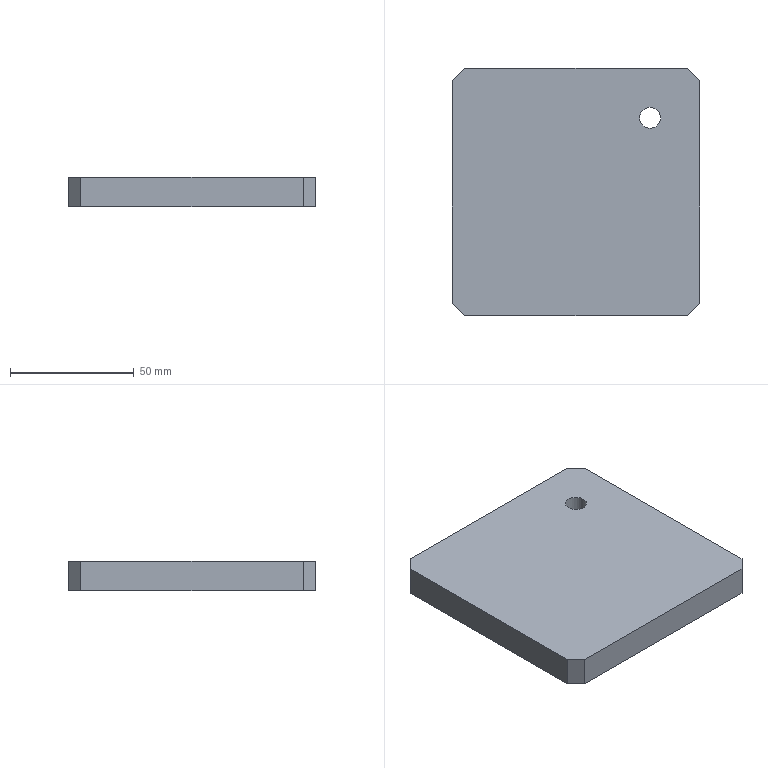Part | NX | features BREP 1 | 1 solid | 11 faces | box 100 x 100 x 12 mm | volume 118719 mm3 | plane 10 | cylinder 1 | commonest cylinder face diameters 8.5 x1
STEP:
#1=CARTESIAN_POINT('',(50.,-45.,12.));
#2=VERTEX_POINT('',#1);
#3=CARTESIAN_POINT('',(50.,45.,12.));
#4=VERTEX_POINT('',#3);
#5=CARTESIAN_POINT('',(50.,-650.,12.));
#6=DIRECTION('',(0.,1.,0.));
#7=VECTOR('',#6,1000.);
#8=LINE('',#5,#7);
#9=EDGE_CURVE('',#2,#4,#8,.T.);
#10=ORIENTED_EDGE('',*,*,#9,.F.);
#11=CARTESIAN_POINT('',(50.,-45.,0.));
#12=VERTEX_POINT('',#11);
#13=CARTESIAN_POINT('',(50.,-45.,15.));
#14=DIRECTION('',(0.,0.,-1.));
#15=VECTOR('',#14,1000.);
#16=LINE('',#13,#15);
#17=EDGE_CURVE('',#2,#12,#16,.T.);
#18=ORIENTED_EDGE('',*,*,#17,.T.);
#19=CARTESIAN_POINT('',(50.,45.,0.));
#20=VERTEX_POINT('',#19);
#21=CARTESIAN_POINT('',(50.,50.,0.));
#22=DIRECTION('',(0.,1.,0.));
#23=VECTOR('',#22,1000.);
#24=LINE('',#21,#23);
#25=EDGE_CURVE('',#12,#20,#24,.T.);
#26=ORIENTED_EDGE('',*,*,#25,.T.);
#27=CARTESIAN_POINT('',(50.,45.,15.));
#28=DIRECTION('',(0.,0.,1.));
#29=VECTOR('',#28,1000.);
#30=LINE('',#27,#29);
#31=EDGE_CURVE('',#20,#4,#30,.T.);
#32=ORIENTED_EDGE('',*,*,#31,.T.);
#33=EDGE_LOOP('',(#10,#18,#26,#32));
#34=FACE_BOUND('',#33,.T.);
#35=CARTESIAN_POINT('',(50.,50.,15.));
#36=DIRECTION('',(-1.,0.,0.));
#37=DIRECTION('',(0.,0.,-1.));
#38=AXIS2_PLACEMENT_3D('',#35,#36,#37);
#39=PLANE('',#38);
#40=ADVANCED_FACE('',(#34),#39,.F.);
#41=CARTESIAN_POINT('',(-45.,50.,12.));
#42=VERTEX_POINT('',#41);
#43=CARTESIAN_POINT('',(45.,50.,12.));
#44=VERTEX_POINT('',#43);
#45=CARTESIAN_POINT('',(-1850.,50.,12.));
#46=DIRECTION('',(1.,0.,0.));
#47=VECTOR('',#46,1000.);
#48=LINE('',#45,#47);
#49=EDGE_CURVE('',#42,#44,#48,.T.);
#50=ORIENTED_EDGE('',*,*,#49,.T.);
#51=CARTESIAN_POINT('',(45.,50.,0.));
#52=VERTEX_POINT('',#51);
#53=CARTESIAN_POINT('',(45.,50.,15.));
#54=DIRECTION('',(0.,0.,-1.));
#55=VECTOR('',#54,1000.);
#56=LINE('',#53,#55);
#57=EDGE_CURVE('',#44,#52,#56,.T.);
#58=ORIENTED_EDGE('',*,*,#57,.T.);
#59=CARTESIAN_POINT('',(-45.,50.,0.));
#60=VERTEX_POINT('',#59);
#61=CARTESIAN_POINT('',(-50.,50.,0.));
#62=DIRECTION('',(-1.,0.,0.));
#63=VECTOR('',#62,1000.);
#64=LINE('',#61,#63);
#65=EDGE_CURVE('',#52,#60,#64,.T.);
#66=ORIENTED_EDGE('',*,*,#65,.T.);
#67=CARTESIAN_POINT('',(-45.,50.,15.));
#68=DIRECTION('',(0.,0.,1.));
#69=VECTOR('',#68,1000.);
#70=LINE('',#67,#69);
#71=EDGE_CURVE('',#60,#42,#70,.T.);
#72=ORIENTED_EDGE('',*,*,#71,.T.);
#73=EDGE_LOOP('',(#50,#58,#66,#72));
#74=FACE_BOUND('',#73,.T.);
#75=CARTESIAN_POINT('',(-50.,50.,15.));
#76=DIRECTION('',(0.,-1.,0.));
#77=DIRECTION('',(0.,0.,1.));
#78=AXIS2_PLACEMENT_3D('',#75,#76,#77);
#79=PLANE('',#78);
#80=ADVANCED_FACE('',(#74),#79,.F.);
#81=CARTESIAN_POINT('',(-50.,45.,12.));
#82=VERTEX_POINT('',#81);
#83=CARTESIAN_POINT('',(-50.,-45.,12.));
#84=VERTEX_POINT('',#83);
#85=CARTESIAN_POINT('',(-50.,50.,12.));
#86=DIRECTION('',(0.,-1.,0.));
#87=VECTOR('',#86,1000.);
#88=LINE('',#85,#87);
#89=EDGE_CURVE('',#82,#84,#88,.T.);
#90=ORIENTED_EDGE('',*,*,#89,.F.);
#91=CARTESIAN_POINT('',(-50.,45.,0.));
#92=VERTEX_POINT('',#91);
#93=CARTESIAN_POINT('',(-50.,45.,15.));
#94=DIRECTION('',(0.,0.,-1.));
#95=VECTOR('',#94,1000.);
#96=LINE('',#93,#95);
#97=EDGE_CURVE('',#82,#92,#96,.T.);
#98=ORIENTED_EDGE('',*,*,#97,.T.);
#99=CARTESIAN_POINT('',(-50.,-45.,0.));
#100=VERTEX_POINT('',#99);
#101=CARTESIAN_POINT('',(-50.,50.,0.));
#102=DIRECTION('',(0.,-1.,0.));
#103=VECTOR('',#102,1000.);
#104=LINE('',#101,#103);
#105=EDGE_CURVE('',#92,#100,#104,.T.);
#106=ORIENTED_EDGE('',*,*,#105,.T.);
#107=CARTESIAN_POINT('',(-50.,-45.,15.));
#108=DIRECTION('',(0.,0.,1.));
#109=VECTOR('',#108,1000.);
#110=LINE('',#107,#109);
#111=EDGE_CURVE('',#100,#84,#110,.T.);
#112=ORIENTED_EDGE('',*,*,#111,.T.);
#113=EDGE_LOOP('',(#90,#98,#106,#112));
#114=FACE_BOUND('',#113,.T.);
#115=CARTESIAN_POINT('',(-50.,50.,15.));
#116=DIRECTION('',(1.,0.,0.));
#117=DIRECTION('',(0.,-1.,0.));
#118=AXIS2_PLACEMENT_3D('',#115,#116,#117);
#119=PLANE('',#118);
#120=ADVANCED_FACE('',(#114),#119,.F.);
#121=CARTESIAN_POINT('',(-45.,-50.,12.));
#122=VERTEX_POINT('',#121);
#123=CARTESIAN_POINT('',(45.,-50.,12.));
#124=VERTEX_POINT('',#123);
#125=CARTESIAN_POINT('',(-50.,-50.,12.));
#126=DIRECTION('',(1.,0.,0.));
#127=VECTOR('',#126,1000.);
#128=LINE('',#125,#127);
#129=EDGE_CURVE('',#122,#124,#128,.T.);
#130=ORIENTED_EDGE('',*,*,#129,.F.);
#131=CARTESIAN_POINT('',(-45.,-50.,0.));
#132=VERTEX_POINT('',#131);
#133=CARTESIAN_POINT('',(-45.,-50.,15.));
#134=DIRECTION('',(0.,0.,-1.));
#135=VECTOR('',#134,1000.);
#136=LINE('',#133,#135);
#137=EDGE_CURVE('',#122,#132,#136,.T.);
#138=ORIENTED_EDGE('',*,*,#137,.T.);
#139=CARTESIAN_POINT('',(45.,-50.,0.));
#140=VERTEX_POINT('',#139);
#141=CARTESIAN_POINT('',(-50.,-50.,0.));
#142=DIRECTION('',(1.,0.,0.));
#143=VECTOR('',#142,1000.);
#144=LINE('',#141,#143);
#145=EDGE_CURVE('',#132,#140,#144,.T.);
#146=ORIENTED_EDGE('',*,*,#145,.T.);
#147=CARTESIAN_POINT('',(45.,-50.,15.));
#148=DIRECTION('',(0.,0.,1.));
#149=VECTOR('',#148,1000.);
#150=LINE('',#147,#149);
#151=EDGE_CURVE('',#140,#124,#150,.T.);
#152=ORIENTED_EDGE('',*,*,#151,.T.);
#153=EDGE_LOOP('',(#130,#138,#146,#152));
#154=FACE_BOUND('',#153,.T.);
#155=CARTESIAN_POINT('',(-50.,-50.,15.));
#156=DIRECTION('',(0.,1.,0.));
#157=DIRECTION('',(0.,0.,-1.));
#158=AXIS2_PLACEMENT_3D('',#155,#156,#157);
#159=PLANE('',#158);
#160=ADVANCED_FACE('',(#154),#159,.F.);
#161=ORIENTED_EDGE('',*,*,#137,.F.);
#162=CARTESIAN_POINT('',(-45.,-50.,12.));
#163=DIRECTION('',(-0.7071,0.7071,0.));
#164=VECTOR('',#163,1000.);
#165=LINE('',#162,#164);
#166=EDGE_CURVE('',#122,#84,#165,.T.);
#167=ORIENTED_EDGE('',*,*,#166,.T.);
#168=ORIENTED_EDGE('',*,*,#111,.F.);
#169=CARTESIAN_POINT('',(-45.,-50.,0.));
#170=DIRECTION('',(-0.7071,0.7071,0.));
#171=VECTOR('',#170,1000.);
#172=LINE('',#169,#171);
#173=EDGE_CURVE('',#132,#100,#172,.T.);
#174=ORIENTED_EDGE('',*,*,#173,.F.);
#175=EDGE_LOOP('',(#161,#167,#168,#174));
#176=FACE_BOUND('',#175,.T.);
#177=CARTESIAN_POINT('',(-45.,-50.,15.));
#178=DIRECTION('',(0.7071,0.7071,0.));
#179=DIRECTION('',(0.,0.,1.));
#180=AXIS2_PLACEMENT_3D('',#177,#178,#179);
#181=PLANE('',#180);
#182=ADVANCED_FACE('',(#176),#181,.F.);
#183=ORIENTED_EDGE('',*,*,#17,.F.);
#184=CARTESIAN_POINT('',(50.,-45.,12.));
#185=DIRECTION('',(-0.7071,-0.7071,0.));
#186=VECTOR('',#185,1000.);
#187=LINE('',#184,#186);
#188=EDGE_CURVE('',#2,#124,#187,.T.);
#189=ORIENTED_EDGE('',*,*,#188,.T.);
#190=ORIENTED_EDGE('',*,*,#151,.F.);
#191=CARTESIAN_POINT('',(50.,-45.,0.));
#192=DIRECTION('',(-0.7071,-0.7071,0.));
#193=VECTOR('',#192,1000.);
#194=LINE('',#191,#193);
#195=EDGE_CURVE('',#12,#140,#194,.T.);
#196=ORIENTED_EDGE('',*,*,#195,.F.);
#197=EDGE_LOOP('',(#183,#189,#190,#196));
#198=FACE_BOUND('',#197,.T.);
#199=CARTESIAN_POINT('',(50.,-45.,15.));
#200=DIRECTION('',(-0.7071,0.7071,0.));
#201=DIRECTION('',(0.,0.,1.));
#202=AXIS2_PLACEMENT_3D('',#199,#200,#201);
#203=PLANE('',#202);
#204=ADVANCED_FACE('',(#198),#203,.F.);
#205=ORIENTED_EDGE('',*,*,#57,.F.);
#206=CARTESIAN_POINT('',(45.,50.,12.));
#207=DIRECTION('',(0.7071,-0.7071,0.));
#208=VECTOR('',#207,1000.);
#209=LINE('',#206,#208);
#210=EDGE_CURVE('',#44,#4,#209,.T.);
#211=ORIENTED_EDGE('',*,*,#210,.T.);
#212=ORIENTED_EDGE('',*,*,#31,.F.);
#213=CARTESIAN_POINT('',(45.,50.,0.));
#214=DIRECTION('',(0.7071,-0.7071,0.));
#215=VECTOR('',#214,1000.);
#216=LINE('',#213,#215);
#217=EDGE_CURVE('',#52,#20,#216,.T.);
#218=ORIENTED_EDGE('',*,*,#217,.F.);
#219=EDGE_LOOP('',(#205,#211,#212,#218));
#220=FACE_BOUND('',#219,.T.);
#221=CARTESIAN_POINT('',(45.,50.,15.));
#222=DIRECTION('',(-0.7071,-0.7071,0.));
#223=DIRECTION('',(0.,0.,1.));
#224=AXIS2_PLACEMENT_3D('',#221,#222,#223);
#225=PLANE('',#224);
#226=ADVANCED_FACE('',(#220),#225,.F.);
#227=ORIENTED_EDGE('',*,*,#97,.F.);
#228=CARTESIAN_POINT('',(-50.,45.,12.));
#229=DIRECTION('',(0.7071,0.7071,0.));
#230=VECTOR('',#229,1000.);
#231=LINE('',#228,#230);
#232=EDGE_CURVE('',#82,#42,#231,.T.);
#233=ORIENTED_EDGE('',*,*,#232,.T.);
#234=ORIENTED_EDGE('',*,*,#71,.F.);
#235=CARTESIAN_POINT('',(-50.,45.,0.));
#236=DIRECTION('',(0.7071,0.7071,0.));
#237=VECTOR('',#236,1000.);
#238=LINE('',#235,#237);
#239=EDGE_CURVE('',#92,#60,#238,.T.);
#240=ORIENTED_EDGE('',*,*,#239,.F.);
#241=EDGE_LOOP('',(#227,#233,#234,#240));
#242=FACE_BOUND('',#241,.T.);
#243=CARTESIAN_POINT('',(-50.,45.,15.));
#244=DIRECTION('',(0.7071,-0.7071,0.));
#245=DIRECTION('',(0.,0.,1.));
#246=AXIS2_PLACEMENT_3D('',#243,#244,#245);
#247=PLANE('',#246);
#248=ADVANCED_FACE('',(#242),#247,.F.);
#249=CARTESIAN_POINT('',(34.25,30.,0.));
#250=VERTEX_POINT('',#249);
#251=CARTESIAN_POINT('',(30.,30.,0.));
#252=DIRECTION('',(0.,0.,1.));
#253=DIRECTION('',(1.,0.,0.));
#254=AXIS2_PLACEMENT_3D('',#251,#252,#253);
#255=CIRCLE('',#254,4.25);
#256=EDGE_CURVE('',#250,#250,#255,.T.);
#257=ORIENTED_EDGE('',*,*,#256,.T.);
#258=EDGE_LOOP('',(#257));
#259=FACE_BOUND('',#258,.T.);
#260=ORIENTED_EDGE('',*,*,#145,.F.);
#261=ORIENTED_EDGE('',*,*,#173,.T.);
#262=ORIENTED_EDGE('',*,*,#105,.F.);
#263=ORIENTED_EDGE('',*,*,#239,.T.);
#264=ORIENTED_EDGE('',*,*,#65,.F.);
#265=ORIENTED_EDGE('',*,*,#217,.T.);
#266=ORIENTED_EDGE('',*,*,#25,.F.);
#267=ORIENTED_EDGE('',*,*,#195,.T.);
#268=EDGE_LOOP('',(#260,#261,#262,#263,#264,#265,#266,#267));
#269=FACE_BOUND('',#268,.T.);
#270=CARTESIAN_POINT('',(0.,0.,0.));
#271=DIRECTION('',(0.,0.,1.));
#272=DIRECTION('',(-1.,0.,0.));
#273=AXIS2_PLACEMENT_3D('',#270,#271,#272);
#274=PLANE('',#273);
#275=ADVANCED_FACE('',(#259,#269),#274,.F.);
#276=CARTESIAN_POINT('',(34.25,30.,12.));
#277=VERTEX_POINT('',#276);
#278=CARTESIAN_POINT('',(30.,30.,12.));
#279=DIRECTION('',(0.,0.,1.));
#280=DIRECTION('',(1.,0.,0.));
#281=AXIS2_PLACEMENT_3D('',#278,#279,#280);
#282=CIRCLE('',#281,4.25);
#283=EDGE_CURVE('',#277,#277,#282,.T.);
#284=ORIENTED_EDGE('',*,*,#283,.F.);
#285=EDGE_LOOP('',(#284));
#286=FACE_BOUND('',#285,.T.);
#287=ORIENTED_EDGE('',*,*,#49,.F.);
#288=ORIENTED_EDGE('',*,*,#232,.F.);
#289=ORIENTED_EDGE('',*,*,#89,.T.);
#290=ORIENTED_EDGE('',*,*,#166,.F.);
#291=ORIENTED_EDGE('',*,*,#129,.T.);
#292=ORIENTED_EDGE('',*,*,#188,.F.);
#293=ORIENTED_EDGE('',*,*,#9,.T.);
#294=ORIENTED_EDGE('',*,*,#210,.F.);
#295=EDGE_LOOP('',(#287,#288,#289,#290,#291,#292,#293,#294));
#296=FACE_BOUND('',#295,.T.);
#297=CARTESIAN_POINT('',(-900.,-300.,12.));
#298=DIRECTION('',(0.,0.,1.));
#299=DIRECTION('',(-1.,0.,0.));
#300=AXIS2_PLACEMENT_3D('',#297,#298,#299);
#301=PLANE('',#300);
#302=ADVANCED_FACE('',(#286,#296),#301,.T.);
#303=ORIENTED_EDGE('',*,*,#283,.T.);
#304=EDGE_LOOP('',(#303));
#305=FACE_BOUND('',#304,.T.);
#306=ORIENTED_EDGE('',*,*,#256,.F.);
#307=EDGE_LOOP('',(#306));
#308=FACE_BOUND('',#307,.T.);
#309=CARTESIAN_POINT('',(30.,30.,12.));
#310=DIRECTION('',(0.,0.,1.));
#311=DIRECTION('',(-1.,0.,0.));
#312=AXIS2_PLACEMENT_3D('',#309,#310,#311);
#313=CYLINDRICAL_SURFACE('',#312,4.25);
#314=ADVANCED_FACE('',(#305,#308),#313,.F.);
#315=CLOSED_SHELL('',(#40,#80,#120,#160,#182,#204,#226,#248,#275,#302,#314));
#316=MANIFOLD_SOLID_BREP('',#315);
#317=(LENGTH_UNIT()NAMED_UNIT(*)SI_UNIT(.MILLI.,.METRE.));
#318=UNCERTAINTY_MEASURE_WITH_UNIT(LENGTH_MEASURE(0.00001),#317,'','');
#319=(NAMED_UNIT(*)PLANE_ANGLE_UNIT()SI_UNIT($,.RADIAN.));
#320=(NAMED_UNIT(*)SI_UNIT($,.STERADIAN.)SOLID_ANGLE_UNIT());
#321=(GEOMETRIC_REPRESENTATION_CONTEXT(3)GLOBAL_UNCERTAINTY_ASSIGNED_CONTEXT((#318))GLOBAL_UNIT_ASSIGNED_CONTEXT((#317,#319,#320))REPRESENTATION_CONTEXT('',''));
#322=ADVANCED_BREP_SHAPE_REPRESENTATION('',(#316),#321);